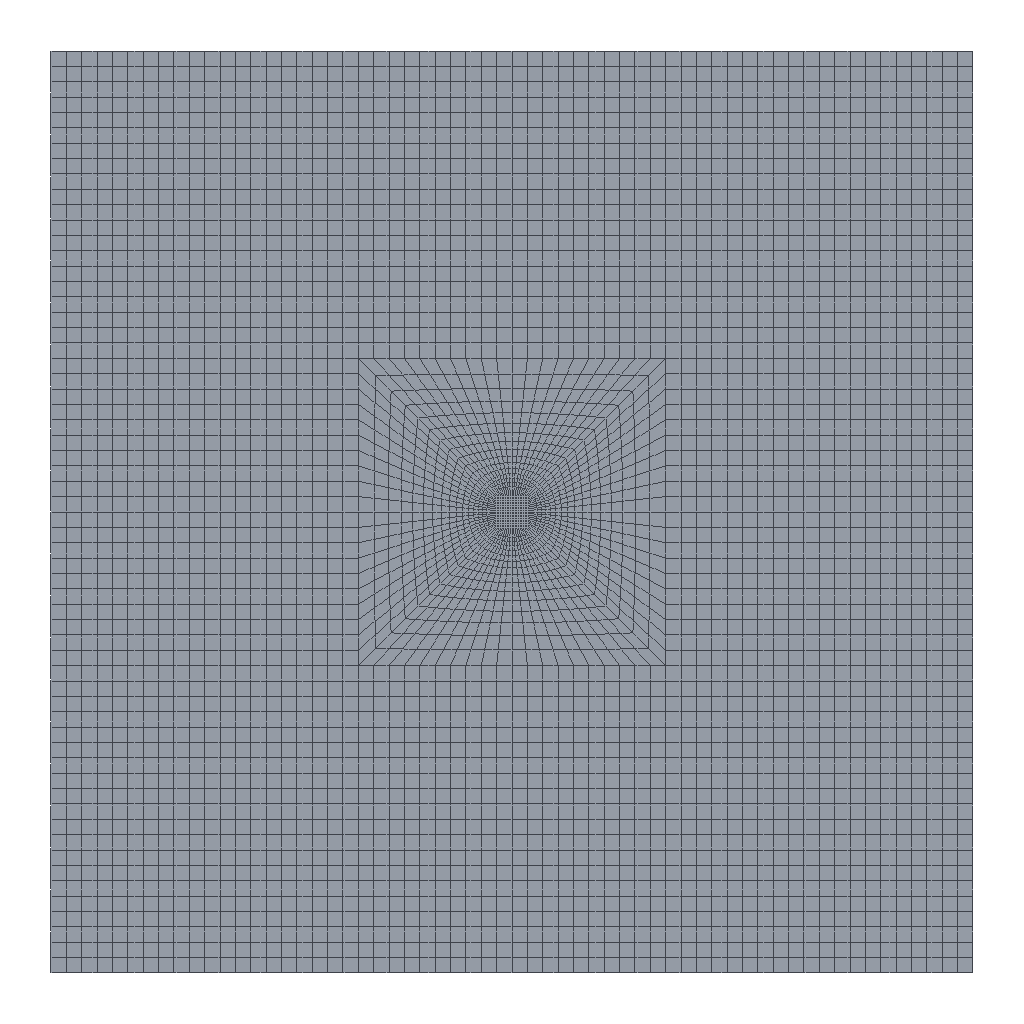Simulation study | abaqus
Set-up summary:
category,name,step,type,value,unit,region
solver,abaqus
solver,version,,,Abaqus/Standard 2020
units,not stated in the deck,,not stated
analysis,deck,,geostatic,geostatic
load_step,Step-1-GEO,Step-1-GEO,geostatic,nlgeom=False
contact,interactions,,,general=0 pairs=0 ties=0
load_step,requested,,,1
mesh,nodes,,,5081
mesh,elements,,,4960
element_type,CPE4RP,,plane,4960
load,load commands in deck,,count,3
bc,support commands in deck,,count,4
material,ROCK,,in results
check,setup vs results,,match,"per instance, exact: element labels, types and connectivity; labels of the nodes the elements use; coordinates of those nodes at SINGLE_PRECISION in 1 of 1 instance(s)"
Abaqus input file, long lists of numbers shortened:
*Heading
** Job name: Job-1 Model name: Model-1
** Generated by: Abaqus/CAE 2020
*Preprint, echo=NO, model=NO, history=NO, contact=NO
**
** PARTS
**
*Part, name=ROCK
*Node
      1,   1.06,   1.06
      2,   1.768,   1.768
** (5079 more lines like these left out)
*Element, type=CPE4RP
 1,   1,  37, 753,  62
 2,  37,  38, 754, 753
** (4958 more lines like these left out)
*Nset, nset=Set-ALLROCK, generate
    1,  5081,     1
*Elset, elset=Set-ALLROCK, generate
    1,  4960,     1
*Nset, nset=Set-CL-ZHONGJIAN
    1,    2,    3,    4,    5,    6,    7,    8,    9,   10,   11,   12,   13,   14,   15,   16
   17,   18,   22,   23,   26,   27,   28,   33,   37,   38,   39,   40,   41,   42,   43,   44
** (111 more lines like these left out)
*Elset, elset=Set-CL-ZHONGJIAN
    1,    2,    3,    4,    5,    6,    7,    8,    9,   10,   11,   12,   13,   14,   15,   16
   17,   18,   19,   20,   21,   22,   23,   24,   25,   26,   27,   28,   29,   30,   31,   32
** (108 more lines like these left out)
*Nset, nset=Set-CL-SUIDONG
    1,    2,    3,    4,    5,    6,    7,    8,    9,   10,   11,   12,   13,   14,   15,   16
   37,   38,   39,   40,   41,   42,   43,   44,   45,   46,   47,   48,   49,   50,   51,   52
** (51 more lines like these left out)
*Elset, elset=Set-CL-SUIDONG
    1,    2,    3,    4,    5,    6,    7,    8,    9,   10,   11,   12,   13,   14,   15,   16
   17,   18,   19,   20,   21,   22,   23,   24,   25,   26,   27,   28,   29,   30,   31,   32
** (48 more lines like these left out)
*Nset, nset=Set-zuoshang
   17,   19,   20,   21,  244,  245,  246,  247,  248,  249,  250,  251,  252,  253,  254,  255
  256,  257,  258,  259,  260,  261,  262,  263,  264,  265,  266,  267,  268,  269,  270,  271
** (26 more lines like these left out)
*Elset, elset=Set-zuoshang, generate
 521,  920,    1
*Nset, nset=Set-zhongshang
   17,   18,   20,   23,   24,  235,  236,  237,  238,  239,  240,  241,  242,  243,  263,  264
  265,  266,  267,  268,  269,  270,  271,  272,  273,  274,  275,  276,  277,  278,  279,  280
** (26 more lines like these left out)
*Elset, elset=Set-zhongshang, generate
 1161,  1560,     1
*Nset, nset=Set-youshang
   23,   24,   29,   30,  360,  361,  362,  363,  364,  365,  366,  367,  368,  369,  370,  371
  372,  373,  374,  375,  376,  377,  378,  496,  497,  498,  499,  500,  501,  502,  503,  504
** (26 more lines like these left out)
*Elset, elset=Set-youshang, generate
 2321,  2720,     1
*Nset, nset=Set-zuozhong
   17,   19,   22,   25,   26,  244,  245,  246,  247,  248,  249,  250,  251,  252,  253,  254
  255,  256,  257,  258,  259,  260,  261,  262,  331,  332,  333,  334,  335,  336,  337,  338
** (26 more lines like these left out)
*Elset, elset=Set-zuozhong, generate
 1561,  1960,     1
*Nset, nset=Set-youzhong
   23,   27,   28,   29,   34,  467,  468,  469,  470,  471,  472,  473,  474,  475,  487,  488
  489,  490,  491,  492,  493,  494,  495,  496,  497,  498,  499,  500,  501,  502,  503,  504
** (26 more lines like these left out)
*Elset, elset=Set-youzhong, generate
 3361,  3760,     1
*Nset, nset=Set-zuoxia
   25,   26,   31,   32,  398,  399,  400,  401,  402,  403,  404,  405,  406,  407,  408,  409
  410,  411,  412,  413,  414,  415,  416,  553,  554,  555,  556,  557,  558,  559,  560,  561
** (26 more lines like these left out)
*Elset, elset=Set-zuoxia, generate
 2721,  3120,     1
*Nset, nset=Set-zhongxia
   26,   27,   32,   33,   35,  591,  592,  593,  594,  595,  596,  597,  598,  599,  600,  601
  602,  603,  604,  605,  606,  607,  608,  609,  621,  622,  623,  624,  625,  626,  627,  628
** (26 more lines like these left out)
*Elset, elset=Set-zhongxia, generate
 3761,  4160,     1
*Nset, nset=Set-youxia
   27,   34,   35,   36,  639,  640,  641,  642,  643,  644,  645,  646,  647,  648,  649,  650
  651,  652,  653,  654,  655,  656,  657,  677,  678,  679,  680,  681,  682,  683,  684,  685
** (26 more lines like these left out)
*Elset, elset=Set-youxia, generate
 4161,  4560,     1
** Section: ROCK
*Solid Section, elset=Set-ALLROCK, material=ROCK
,
*End Part
**
**
** ASSEMBLY
**
*Assembly, name=Assembly
**
*Instance, name=ROCK-1, part=ROCK
*End Instance
**
*Nset, nset=Set-1-ALLROCK, instance=ROCK-1, generate
    1,  5081,     1
*Elset, elset=Set-1-ALLROCK, instance=ROCK-1, generate
    1,  4960,     1
*Nset, nset=Set-2-REMOVE, instance=ROCK-1
    1,    2,    3,    4,    5,    6,    7,    8,    9,   10,   11,   12,   13,   14,   15,   16
   37,   38,   39,   40,   41,   42,   43,   44,   45,   46,   47,   48,   49,   50,   51,   52
** (51 more lines like these left out)
*Elset, elset=Set-2-REMOVE, instance=ROCK-1
    1,    2,    3,    4,    5,    6,    7,    8,    9,   10,   11,   12,   13,   14,   15,   16
   17,   18,   19,   20,   21,   22,   23,   24,   25,   26,   27,   28,   29,   30,   31,   32
** (48 more lines like these left out)
*Nset, nset=Set-3-ZHONGJIAN, instance=ROCK-1
    1,    2,    3,    4,    5,    6,    7,    8,    9,   10,   11,   12,   13,   14,   15,   16
   17,   18,   22,   23,   26,   27,   28,   33,   37,   38,   39,   40,   41,   42,   43,   44
** (111 more lines like these left out)
*Elset, elset=Set-3-ZHONGJIAN, instance=ROCK-1
    1,    2,    3,    4,    5,    6,    7,    8,    9,   10,   11,   12,   13,   14,   15,   16
   17,   18,   19,   20,   21,   22,   23,   24,   25,   26,   27,   28,   29,   30,   31,   32
** (108 more lines like these left out)
*Nset, nset=Set-4-BOTTOM, instance=ROCK-1
  31,  32,  35,  36, 572, 573, 574, 575, 576, 577, 578, 579, 580, 581, 582, 583
 584, 585, 586, 587, 588, 589, 590, 696, 697, 698, 699, 700, 701, 702, 703, 704
** (2 more lines like these left out)
*Nset, nset=Set-5-LEFT, instance=ROCK-1
  19,  21,  25,  31, 301, 302, 303, 304, 305, 306, 307, 308, 309, 310, 311, 312
 313, 314, 315, 316, 317, 318, 319, 426, 427, 428, 429, 430, 431, 432, 433, 434
** (2 more lines like these left out)
*Nset, nset=Set-6-RIGHT, instance=ROCK-1
  29,  30,  34,  36, 515, 516, 517, 518, 519, 520, 521, 522, 523, 524, 525, 526
 527, 528, 529, 530, 531, 532, 533, 658, 659, 660, 661, 662, 663, 664, 665, 666
** (2 more lines like these left out)
*Nset, nset=Set-7-LIULIANG, instance=ROCK-1
   2,   3,   6,   8,  10,  12,  14,  16,  41,  42,  43,  44,  45,  46,  47,  48
  49,  67,  68,  69,  70,  71,  72,  73,  74,  75,  89,  90,  91,  92,  93,  94
** (3 more lines like these left out)
*Nset, nset=Set-8-NODES, instance=ROCK-1
  3,  6, 10, 14
*Nset, nset=Set-9-TOP, instance=ROCK-1
  20,  21,  24,  30, 282, 283, 284, 285, 286, 287, 288, 289, 290, 291, 292, 293
 294, 295, 296, 297, 298, 299, 300, 379, 380, 381, 382, 383, 384, 385, 386, 387
** (2 more lines like these left out)
*Nset, nset=Set-11, instance=ROCK-1
  19,  21,  25,  29,  30,  31,  34,  36, 301, 302, 303, 304, 305, 306, 307, 308
 309, 310, 311, 312, 313, 314, 315, 316, 317, 318, 319, 426, 427, 428, 429, 430
** (6 more lines like these left out)
*Elset, elset=Set-11, instance=ROCK-1
  521,  541,  561,  581,  601,  621,  641,  661,  681,  701,  721,  741,  761,  781,  801,  821
  841,  861,  881,  901, 1561, 1581, 1601, 1621, 1641, 1661, 1681, 1701, 1721, 1741, 1761, 1781
** (6 more lines like these left out)
*Nset, nset=Set-12, instance=ROCK-1
  31,  32,  35,  36, 572, 573, 574, 575, 576, 577, 578, 579, 580, 581, 582, 583
 584, 585, 586, 587, 588, 589, 590, 696, 697, 698, 699, 700, 701, 702, 703, 704
** (2 more lines like these left out)
*Elset, elset=Set-12, instance=ROCK-1
 3101, 3102, 3103, 3104, 3105, 3106, 3107, 3108, 3109, 3110, 3111, 3112, 3113, 3114, 3115, 3116
 3117, 3118, 3119, 3120, 3761, 3781, 3801, 3821, 3841, 3861, 3881, 3901, 3921, 3941, 3961, 3981
** (2 more lines like these left out)
*Nset, nset=Set-13, instance=ROCK-1
   2,   3,   6,   8,  10,  12,  14,  16,  41,  42,  43,  44,  45,  46,  47,  48
  49,  67,  68,  69,  70,  71,  72,  73,  74,  75,  89,  90,  91,  92,  93,  94
** (3 more lines like these left out)
*Elset, elset=Set-13, instance=ROCK-1
    5,   10,   15,   20,   25,   30,   35,   40,   45,   50,   55,   60,   65,   70,   75,   80
   85,   90,   95,  100,  105,  110,  115,  120,  125,  130,  135,  140,  145,  150,  155,  160
** (8 more lines like these left out)
*Nset, nset=Set-14, instance=ROCK-1, generate
    1,  5081,     1
*Elset, elset=Set-14, instance=ROCK-1, generate
    1,  4960,     1
*Nset, nset=Set-15, instance=ROCK-1
  20,  21,  24,  30, 282, 283, 284, 285, 286, 287, 288, 289, 290, 291, 292, 293
 294, 295, 296, 297, 298, 299, 300, 379, 380, 381, 382, 383, 384, 385, 386, 387
** (2 more lines like these left out)
*Elset, elset=Set-15, instance=ROCK-1
  901,  902,  903,  904,  905,  906,  907,  908,  909,  910,  911,  912,  913,  914,  915,  916
  917,  918,  919,  920, 1180, 1200, 1220, 1240, 1260, 1280, 1300, 1320, 1340, 1360, 1380, 1400
** (2 more lines like these left out)
*Nset, nset=Set-16, instance=ROCK-1
  20,  21,  24,  30, 282, 283, 284, 285, 286, 287, 288, 289, 290, 291, 292, 293
 294, 295, 296, 297, 298, 299, 300, 379, 380, 381, 382, 383, 384, 385, 386, 387
** (2 more lines like these left out)
*Elset, elset=Set-16, instance=ROCK-1
  901,  902,  903,  904,  905,  906,  907,  908,  909,  910,  911,  912,  913,  914,  915,  916
  917,  918,  919,  920, 1180, 1200, 1220, 1240, 1260, 1280, 1300, 1320, 1340, 1360, 1380, 1400
** (2 more lines like these left out)
*Nset, nset=Set-ALLNODES, instance=ROCK-1, generate
    1,  5081,     1
*Elset, elset=_Surf-1-TOP_S3, internal, instance=ROCK-1, generate
 901,  920,    1
*Elset, elset=_Surf-1-TOP_S2, internal, instance=ROCK-1, generate
 1180,  1560,    20
*Elset, elset=_Surf-1-TOP_S4, internal, instance=ROCK-1, generate
 2321,  2701,    20
*Surface, type=ELEMENT, name=Surf-1-TOP
_Surf-1-TOP_S3, S3
_Surf-1-TOP_S2, S2
_Surf-1-TOP_S4, S4
*Elset, elset=_Surf-2_S3, internal, instance=ROCK-1, generate
 901,  920,    1
*Elset, elset=_Surf-2_S2, internal, instance=ROCK-1, generate
 1180,  1560,    20
*Elset, elset=_Surf-2_S4, internal, instance=ROCK-1, generate
 2321,  2701,    20
*Surface, type=ELEMENT, name=Surf-2
_Surf-2_S3, S3
_Surf-2_S2, S2
_Surf-2_S4, S4
*Nset, nset=Set-16_PP_, internal, instance=ROCK-1
  20,  21,  24,  30, 282, 283, 284, 285, 286, 287, 288, 289, 290, 291, 292, 293
 294, 295, 296, 297, 298, 299, 300, 379, 380, 381, 382, 383, 384, 385, 386, 387
** (2 more lines like these left out)
*Nset, nset=Set-13_PP_, internal, instance=ROCK-1
   2,   3,   6,   8,  10,  12,  14,  16,  41,  42,  43,  44,  45,  46,  47,  48
  49,  67,  68,  69,  70,  71,  72,  73,  74,  75,  89,  90,  91,  92,  93,  94
** (3 more lines like these left out)
*End Assembly
*Amplitude, name=Amp-1
             0.,              1.,              1.,              0.
**
** MATERIALS
**
*Material, name=ROCK
*Density
2300.,
*Elastic
 5e+09, 0.3
*Permeability, specific=10000.
 3e-07, 0.16
*Mohr Coulomb
35.,0.
*Mohr Coulomb Hardening
500000.,0.
**
** PREDEFINED FIELDS
**
** Name: Predefined Field-1-POR   Type: Pore pressure
*Initial Conditions, TYPE=PORE PRESSURE
Set-ALLNODES, 2.35e+06, -30., 1.75e+06, 30.
** Name: Predefined Field-2-RATIO   Type: Void ratio
*Initial Conditions, TYPE=RATIO
Set-1-ALLROCK, 0.16
** Name: Predefined Field-3-SAT   Type: Saturation
*Initial Conditions, type=SATURATION
Set-1-ALLROCK, 1.
** Name: Predefined Field-s   Type: Stress
*Initial Conditions, type=STRESS, file=D:/shenliu/model/Job-geo.odb, step=1, inc=1
** ----------------------------------------------------------------
**
** STEP: Step-1-GEO
**
*Step, name=Step-1-GEO, nlgeom=NO, inc=1000, unsymm=YES
*Geostatic, utol=0.01
0.01, 1., 1e-05, 1.
**
** BOUNDARY CONDITIONS
**
** Name: BC-4 Type: 孔隙压力
*Boundary, amplitude=Amp-1
Set-16_PP_, 8, 8, 1.75e+06
** Name: BC-5-LIULIANG Type: 孔隙压力
*Boundary
Set-13_PP_, 8, 8
** Name: [REDACTED] : Displacement/rotation angle
*Boundary
Set-11, 1, 1
** Name: [REDACTED] : Displacement/rotation angle
*Boundary
Set-12, 2, 2
**
** LOADS
**
** Name: Load-1   Type: Gravity
*Dload
, GRAV, 10., 0., -1.
** Name: Load-p   Type: Pressure
*Dsload
Surf-2, P, 4.025e+06
**
** INTERACTIONS
**
** Interaction: Int-1
*Model Change, remove
Set-2-REMOVE,
**
** OUTPUT REQUESTS
**
*Restart, write, frequency=0
**
** FIELD OUTPUT: F-Output-1
**
*Output, field
*Node Output
COORD, POR, RF, RM, RT, RVF, U, V
*Element Output, directions=YES
E, FLUVR, FLVEL, GELVR, LE, MISES, MISESMAX, MISESONLY, NE, PE, PEEQ, PEEQMAX, PEEQT, PEMAG, PEQC, S
SAT, SDV, SEQUT, SSAVG, VOIDR, YIELDPOT
**
** HISTORY OUTPUT: H-Output-1
**
*Output, history, variable=PRESELECT
*End Step
Results summary:
result,step,,completed,increments=11 time=1.0/1.0
result,analysis,,,geostatic
result,last_loadstep,,,1
result,analysis steps,,count,1
result,primary field,,,U
result,reaction total,,FX,0.125,model units
result,reaction total,,FY,328776517.25,model units
result,reaction total,,FZ,0.0,model units